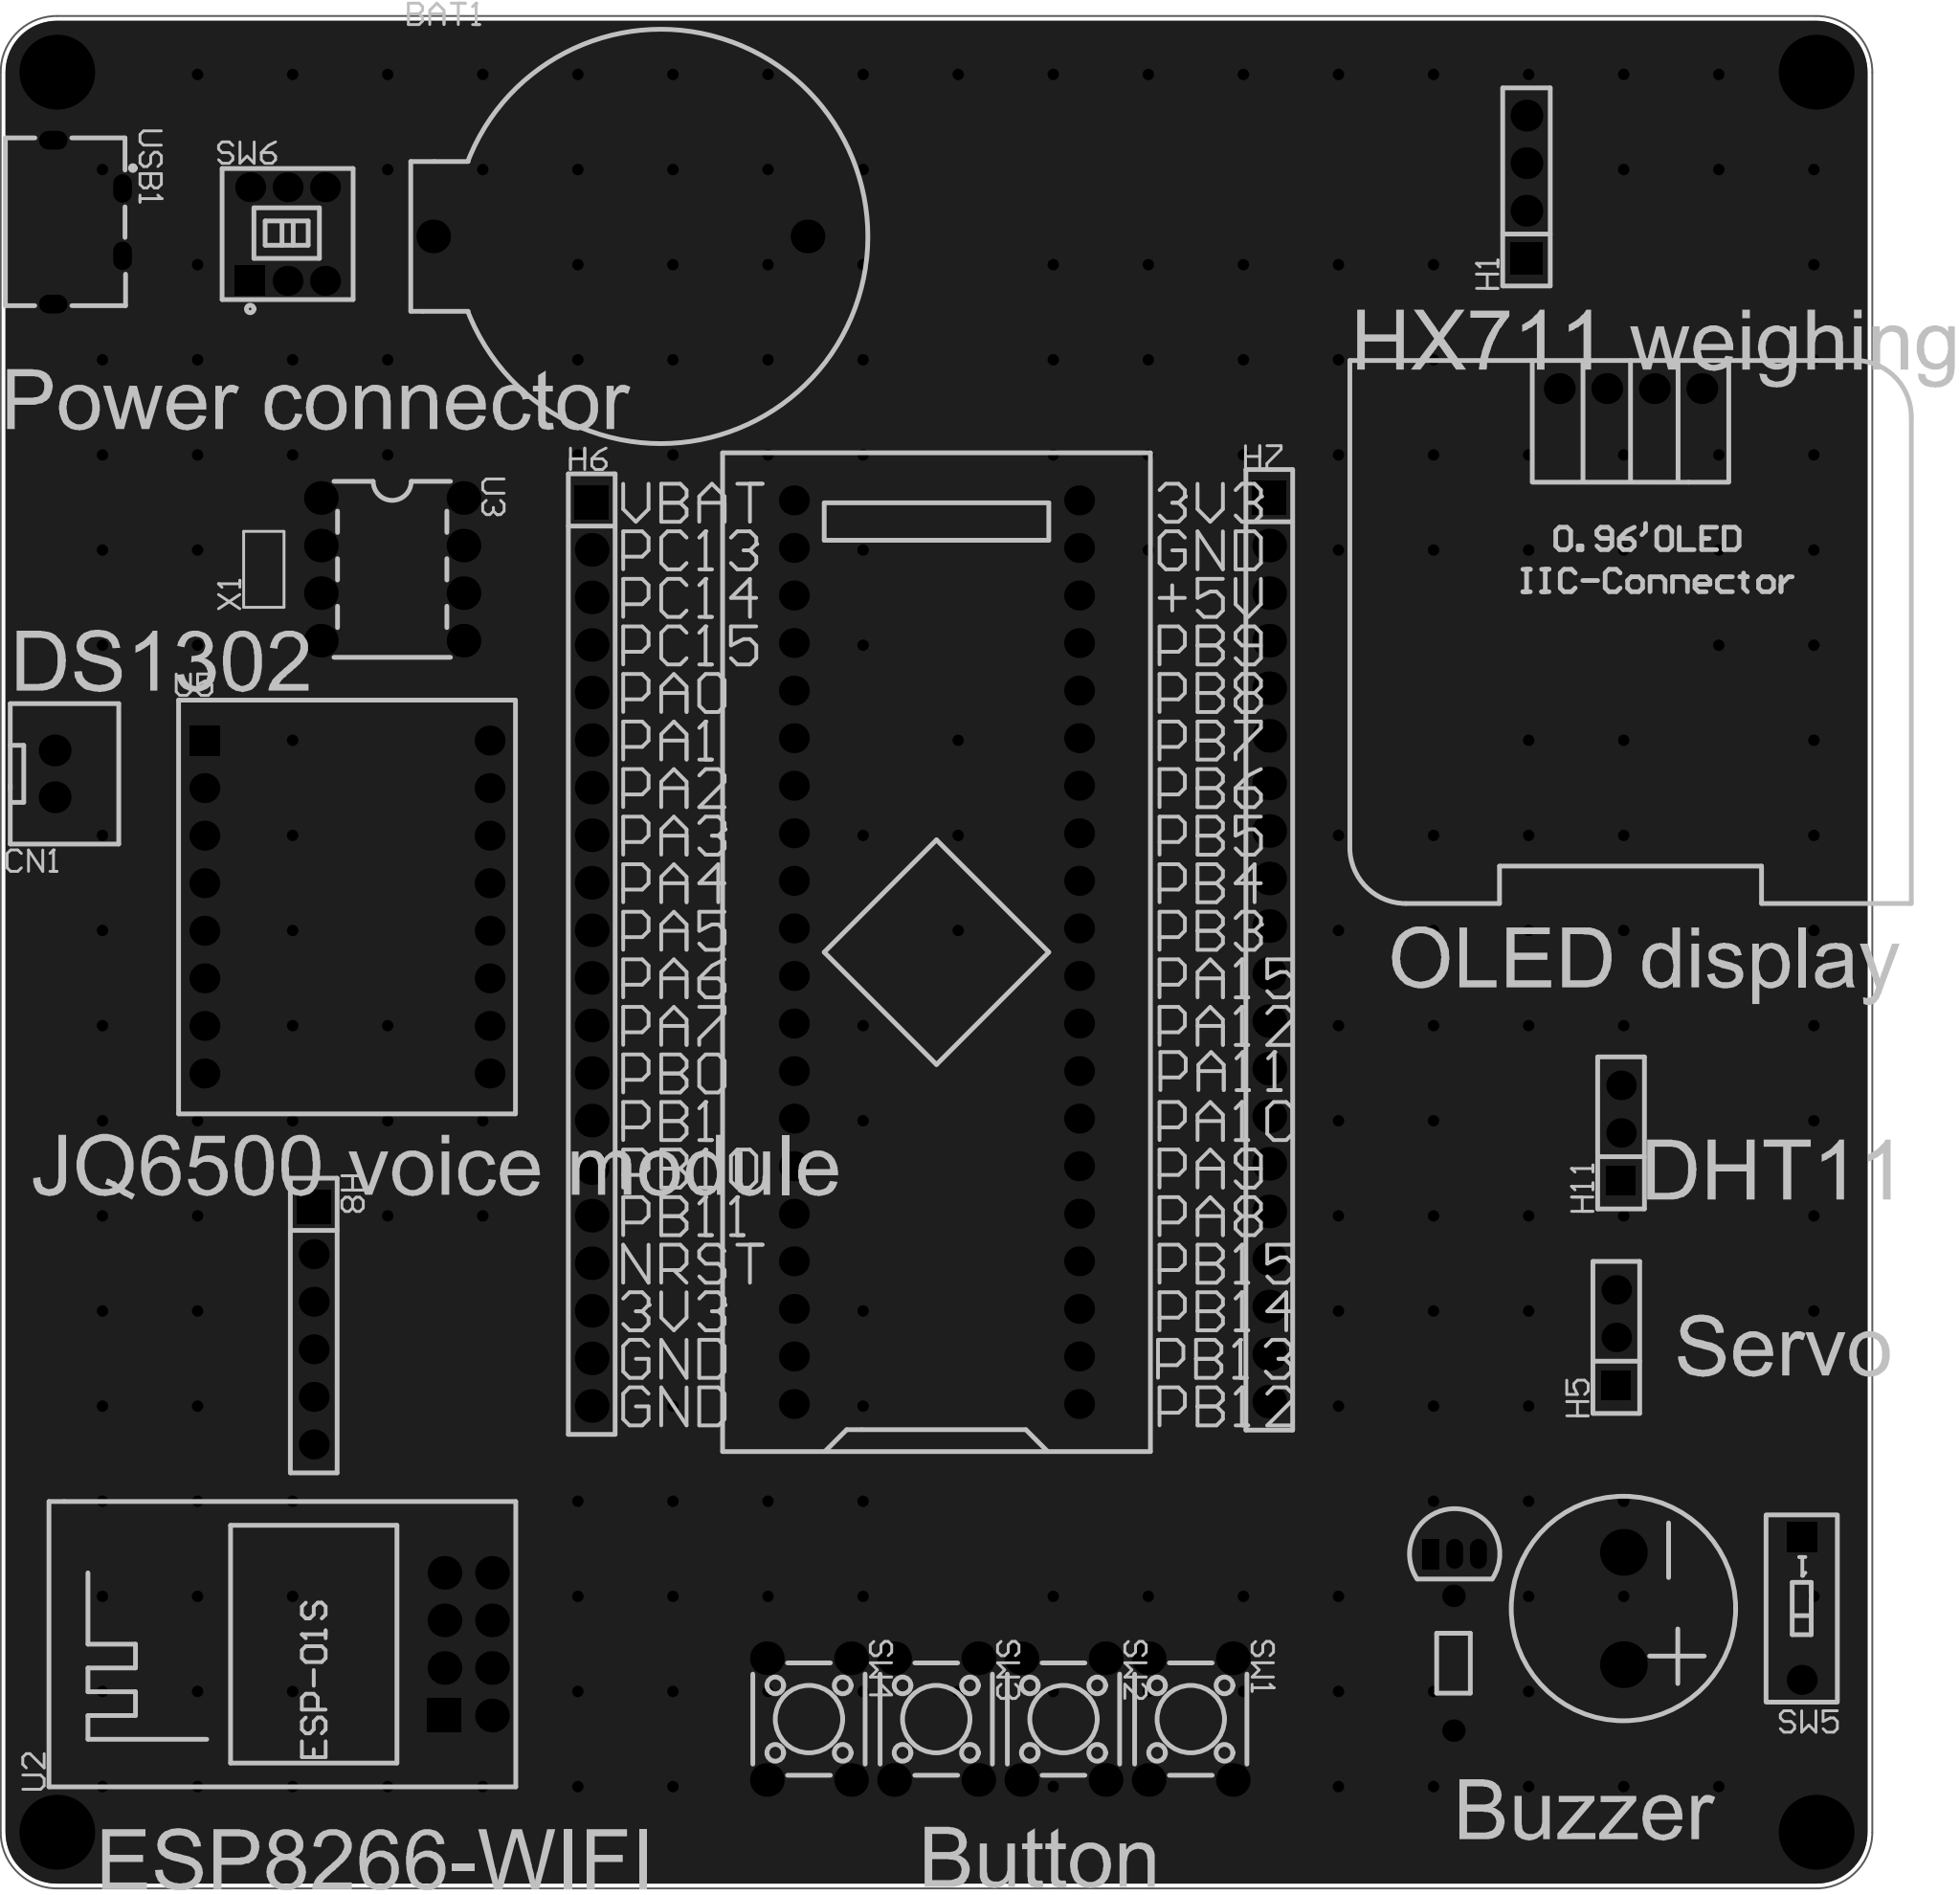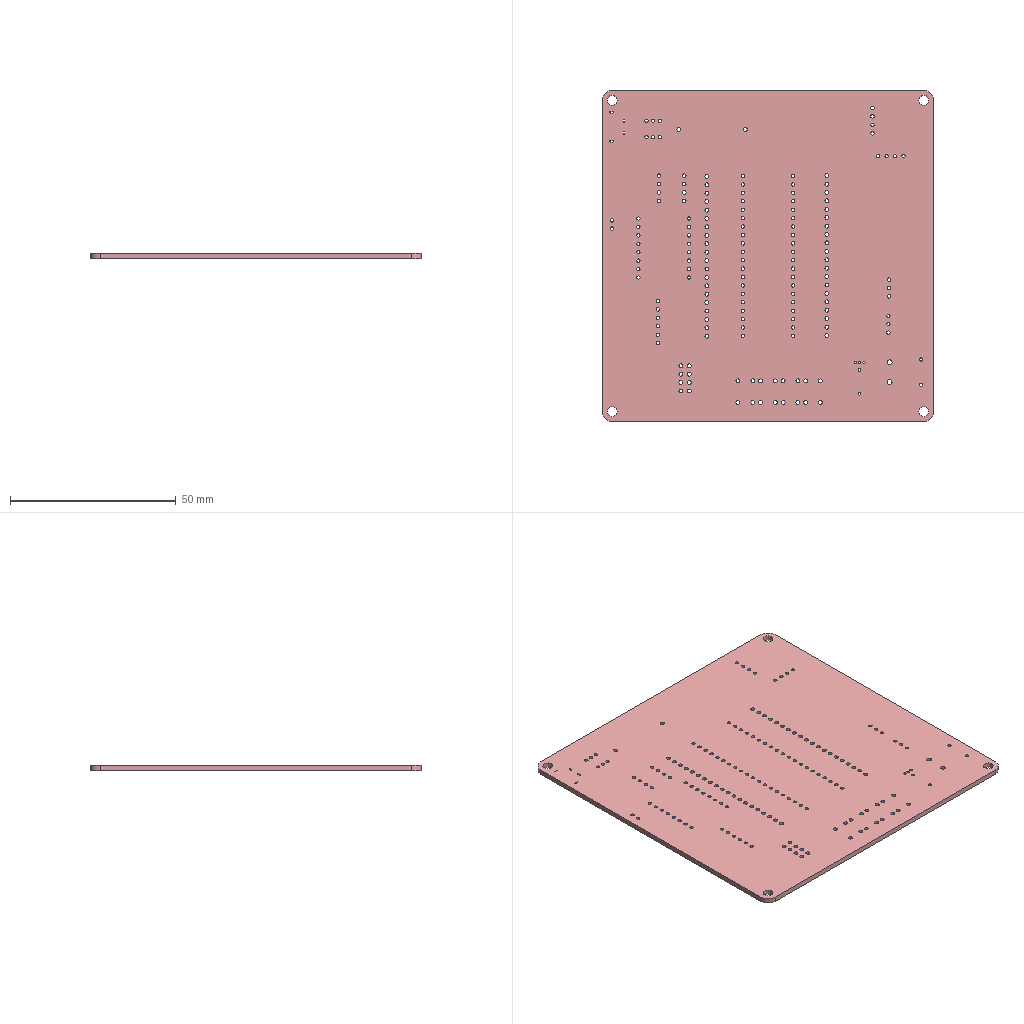Circuit board layout | Altium Designer | box 100 x 100 x 1.6 mm
Layer stack:
# Altium Designer layer stack of  (unit mm; dielectric type: 0 none, 1 core, 2 prepreg, 3 surface material)
index,name,kind,layer,copper_thickness_mm,dielectric_type,dielectric_thickness_mm,dielectric_material,dielectric_constant
0,Top Paste Mask Layer,other,,,,,,
1,Top Silkscreen Layer,other,,,,,,
2,Top Solder Mask Layer,dielectric,,,3,0.01,,3.3
3,Top Layer,copper,Top Layer,0.035,,,,
4,Dielectric1,dielectric,,,3,1.51,FR4,4.5
5,Bottom Layer,copper,Bottom Layer,0.035,,,,
6,Bottom Solder Mask Layer,dielectric,,,3,0.01,,3.3
7,Bottom Silkscreen Layer,other,,,,,,
8,Bottom Paste Mask Layer,other,,,,,,
# drill layer pairs: low layer,high layer
drill_pair,Top Layer,Bottom Layer
Part placement:
Designator,Comment,Layer,Footprint,Center-X(mm),Center-Y(mm),Rotation
U1,STM32F103C8T6-Card,TopLayer,CONN-TH_L53.3-W22.9_STM32F103C8T6-CARD,141.351,130.937,90
OLED1,,TopLayer,0.96OLED_4P,178.435,161.036,0
SW1,,TopLayer,SW-TH_4P-L6.0-W6.0-P4.50-LS6.5,154.936,89.979,270
SW2,,TopLayer,SW-TH_4P-L6.0-W6.0-P4.50-LS6.5,148.136,89.979,270
SW3,,TopLayer,SW-TH_4P-L6.0-W6.0-P4.50-LS6.5,141.337,89.979,270
SW4,,TopLayer,SW-TH_4P-L6.0-W6.0-P4.50-LS6.5,134.537,89.979,270
BAT1,KH-BS2032-2-1,TopLayer,BAT-TH_KH-BS2032-2-1,124.46,169.164,0
CN1,XH2.54*2P_Through-hole,TopLayer,CONN-TH_2P-P2.50-XH2.54-2P,94.234,140.462,90
H1,,TopLayer,HDR-TH_4P-P2.54-V-F,172.873,171.807,90
BUZZER1,buzzer,TopLayer,BUZ-TH_BD12.0-P6.00-D0.9-RD,178.054,95.885,270
R2,1kΩ,TopLayer,Res_1/8W,168.974,92.964,90
H5,,TopLayer,HDR-TH_3P-P2.54-V-F,177.673,110.363,90
H6,,TopLayer,HDR-TH_20P-P2.54-V-F,122.929,130.834,270
H7,,TopLayer,HDR-TH_20P-P2.54-V-F,159.131,131.064,270
H8,,TopLayer,HDR-TH_6P-P2.54-V-F,108.077,110.998,270
H11,,TopLayer,HDR-TH_3P-P2.54-V-F,177.927,121.285,90
Q1,,TopLayer,S8050_TO_92,169.037,98.806,0
SW5,NDS-01V,TopLayer,SW-TH_2P-L3.9-W9.9-P2.54-LS7.6,187.579,95.885,270
SW6,TK-6700-1,TopLayer,SW-TH_TK-6700-1,106.68,169.291,0
U2,ESP-01S,TopLayer,WIFIM-TH_ESP-01S,116.332,93.98,90
U3,DS1302N(XBLW),TopLayer,PDIP-8_L9.3-W6.4-P2.54-LS7.6-BL,112.268,151.384,270
U5,JQ6500,TopLayer,MOD-TH_JQ6500,109.855,133.35,0
USB1,KH-TYPE-C-2P,TopLayer,USB-SMD_KH-TYPE-C-2P,96.012,169.926,270
X1,32.768KHZ,TopLayer,CRYSTAL-SMD_L3.2-W1.5-1,105.41,151.384,90
Pad and via stacks:
# Altium Designer via and pad stacks of  (unit mm). Each distinct definition once, with the count of objects using it.
# via: kind,start_layer,end_layer,hole_mm,diameter_mm,mode(0 simple;1 top-mid-bottom;2 full stack),diameter_per_layer,count,example_net
# pad: kind,layer,hole_mm,hole_type(0 round;1 square;2 slot),plating,top_size,top_shape(1 round;2 rect;3 octagon;9 rounded rect),mid_size,bottom_size,mode,footprint,size_per_layer,count,example
pad,Multi-Layer,3,0,plated,4x4,1,4x4,4x4,0,,,4,1
pad,Multi-Layer,1,0,plated,1.6x1.6,1,1.6x1.6,1.6x1.6,0,CONN-TH_L53.3-W22.9_STM32F103C8T6-CARD,,40,U1.1
pad,Multi-Layer,1,0,plated,1.65x1.65,1,1.65x1.65,1.65x1.65,0,0.96OLED_4P,,4,OLED1.4
pad,Multi-Layer,1.2,0,plated,1.8x1.8,1,1.8x1.8,1.8x1.8,0,SW-TH_4P-L6.0-W6.0-P4.50-LS6.5,,16,SW1.1
pad,Multi-Layer,1.2,0,plated,1.8x1.8,1,1.8x1.8,1.8x1.8,0,BAT-TH_KH-BS2032-2-1,,2,BAT1.1
pad,Multi-Layer,1.05,0,plated,1.7x1.7,1,1.7x1.7,1.7x1.7,0,CONN-TH_2P-P2.50-XH2.54-2P,,2,CN1.2
pad,Multi-Layer,1.1,0,plated,1.7x1.7,2,1.7x1.7,1.7x1.7,0,HDR-TH_4P-P2.54-V-F,,1,H1.1
pad,Multi-Layer,1.1,0,plated,1.7x1.7,1,1.7x1.7,1.7x1.7,0,HDR-TH_4P-P2.54-V-F,,3,H1.2
pad,Multi-Layer,1.5,0,plated,2.5x2.5,1,2.5x2.5,2.5x2.5,0,BUZ-TH_BD12.0-P6.00-D0.9-RD,,2,BUZZER1.1
pad,Multi-Layer,0.8001,0,plated,1.199x1.199,1,1.199x1.199,1.199x1.199,0,Res_1/8W,,2,R2.1
pad,Multi-Layer,1.02,0,plated,1.575x1.575,1,1.575x1.575,1.575x1.575,0,HDR-TH_3P-P2.54-V-F,,4,H5.3
pad,Multi-Layer,1.02,0,plated,1.575x1.575,2,1.575x1.575,1.575x1.575,0,HDR-TH_3P-P2.54-V-F,,2,H5.1
pad,Multi-Layer,1.2,0,plated,1.8x1.8,2,1.8x1.8,1.8x1.8,0,HDR-TH_20P-P2.54-V-F,,2,H6.1
pad,Multi-Layer,1.2,0,plated,1.8x1.8,1,1.8x1.8,1.8x1.8,0,HDR-TH_20P-P2.54-V-F,,38,H6.2
pad,Multi-Layer,1.02,0,plated,1.6x1.6,1,1.6x1.6,1.6x1.6,0,HDR-TH_6P-P2.54-V-F,,5,H8.6
pad,Multi-Layer,1.02,0,plated,1.8x1.8,2,1.8x1.8,1.8x1.8,0,HDR-TH_6P-P2.54-V-F,,1,H8.1
pad,Multi-Layer,0.701,0,plated,0.8992x1.6,2,0.8992x1.6,0.8992x1.6,0,S8050_TO_92,,1,Q1.1
pad,Multi-Layer,0.701,0,plated,0.8992x1.6,1,0.8992x1.6,0.8992x1.6,0,S8050_TO_92,,2,Q1.2
pad,Multi-Layer,1,0,plated,1.6x1.6,2,1.6x1.6,1.6x1.6,0,SW-TH_2P-L3.9-W9.9-P2.54-LS7.6,,1,SW5.1
pad,Multi-Layer,1,0,plated,1.6x1.6,1,1.6x1.6,1.6x1.6,0,SW-TH_2P-L3.9-W9.9-P2.54-LS7.6,,1,SW5.2
pad,Multi-Layer,1,0,plated,1.6x1.6,2,1.6x1.6,1.6x1.6,0,SW-TH_TK-6700-1,,1,SW6.1
pad,Multi-Layer,1,0,plated,1.6x1.6,1,1.6x1.6,1.6x1.6,0,SW-TH_TK-6700-1,,5,SW6.2
pad,Multi-Layer,1.2,0,plated,1.8x1.8,2,1.8x1.8,1.8x1.8,0,WIFIM-TH_ESP-01S,,1,U2.1
pad,Multi-Layer,1.2,0,plated,1.8x1.8,1,1.8x1.8,1.8x1.8,0,WIFIM-TH_ESP-01S,,7,U2.2
pad,Multi-Layer,1.1,0,plated,1.8x1.8,1,1.8x1.8,1.8x1.8,0,PDIP-8_L9.3-W6.4-P2.54-LS7.6-BL,,8,U3.1
pad,Multi-Layer,1,0,plated,1.6x1.6,2,1.6x1.6,1.6x1.6,0,MOD-TH_JQ6500,,1,U5.1
pad,Multi-Layer,1,0,plated,1.6x1.6,1,1.6x1.6,1.6x1.6,0,MOD-TH_JQ6500,,15,U5.2
pad,Multi-Layer,0.45,2,plated,1x1.524,1,1x1.524,1x1.524,0,USB-SMD_KH-TYPE-C-2P,,2,USB1.1
pad,Multi-Layer,0.5,2,plated,1x1.524,1,1x1.524,1x1.524,0,USB-SMD_KH-TYPE-C-2P,,2,USB1.3
pad,Top Layer,0,0,plated,1.05x1.7,2,1.05x1.7,1.05x1.7,0,CRYSTAL-SMD_L3.2-W1.5-1,,2,X1.2
via,Top Layer,Bottom Layer,0.3048,0.61,0,,198,GND
Copper pours:
name,layer,net,type(0 solid;1 hatched;2 none)
Bottom Layer-GND,Bottom Layer,GND,0
Top Layer-GND,Top Layer,GND,0
Design rules, without the lines most boards share:
# Altium Designer design rules of  (exported by Altium Designer, unit mm)
# columns: name | kind | enabled | priority | scope1 | scope2 | descriptor | typed fields (field=value)
Copper_copperRegion_copperThickness1oz | 0 | disabled | 4 | All | All | Clearance Constraint (Gap=5.984mil) (Disabled)(All),(All) | gap=0.152
Copper_copperRegion_copperThickness1oz_1 | 63 | disabled | 4 | All | All | Board Clearance Constraint (Gap=0mil) (Disabled)(All) |
Copper_copperRegion_Copper_copperRegion | 0 | disabled | 5 | All | All | Clearance Constraint (Gap=5.984mil) (Disabled)(All),(All) | gap=0.152
Copper_copperRegion_Copper_copperRegion_1 | 63 | disabled | 5 | All | All | Board Clearance Constraint (Gap=0mil) (Disabled)(All) |
copperThickness1oz | 0 | enabled | 6 | All | All | Clearance Constraint (Gap=5.984mil) (All),(All) | gap=0.152
copperThickness1oz_1 | 63 | enabled | 6 | All | All | Board Clearance Constraint (Gap=0mil) (All) |
copperRegion_copperThickness1oz | 20 | disabled | 1 | All | All | Polygon Connect Rule(Relief Connect )(Conductor Width=10mil) (Relief Angle=90 Angle) (Entries=4) (Air Gap Width=10mil) (Disabled)(All),(All) | connect_style(0=relief,1=direct,2=none)=0 relief_conductor_width=0.254 relief_entries=4
copperRegion_Copper_copperRegion | 20 | disabled | 2 | All | All | Polygon Connect Rule(Relief Connect )(Conductor Width=10mil) (Relief Angle=90 Angle) (Entries=4) (Air Gap Width=10mil) (Disabled)(All),(All) | connect_style(0=relief,1=direct,2=none)=0 relief_conductor_width=0.254 relief_entries=4
copperRegion | 20 | enabled | 3 | All | All | Polygon Connect Rule(Relief Connect )(Conductor Width=10mil) (Relief Angle=90 Angle) (Entries=4) (Air Gap Width=10mil) (All),(All) | connect_style(0=relief,1=direct,2=none)=0 relief_conductor_width=0.254 relief_entries=4